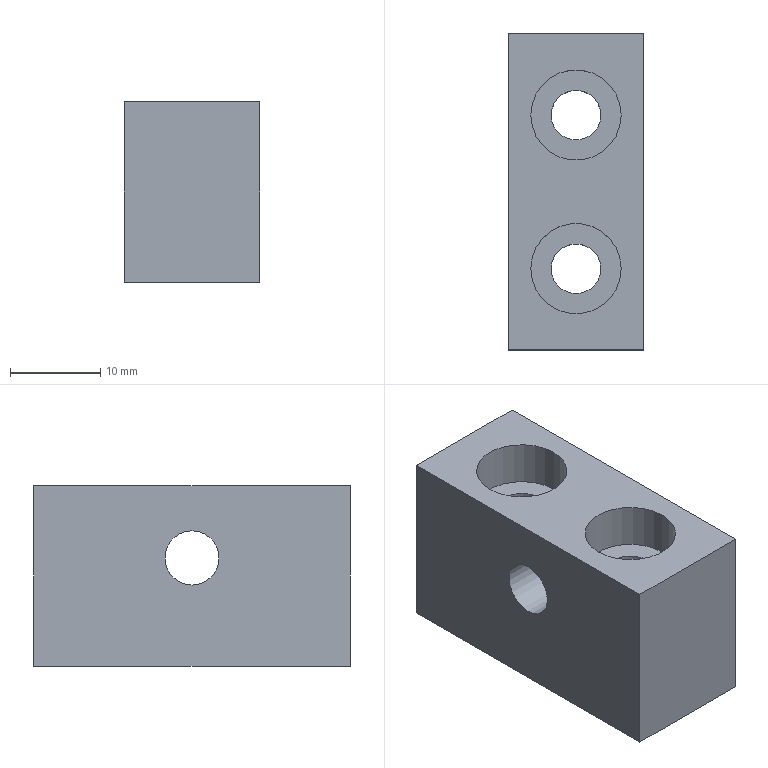Part | NX | features pneumatic support2 2 | 1 solid | 13 faces | box 15 x 35 x 20 mm | volume 8578 mm3 | plane 8 | cylinder 5 | commonest cylinder face diameters 5.5 x2 10 x2 6 x1
STEP:
#1=CARTESIAN_POINT('',(5.,8.5,15.));
#2=VERTEX_POINT('',#1);
#3=CARTESIAN_POINT('',(0.,8.5,15.));
#4=DIRECTION('',(0.,0.,1.));
#5=DIRECTION('',(1.,0.,0.));
#6=AXIS2_PLACEMENT_3D('',#3,#4,#5);
#7=CIRCLE('',#6,5.);
#8=EDGE_CURVE('',#2,#2,#7,.T.);
#9=ORIENTED_EDGE('',*,*,#8,.T.);
#10=EDGE_LOOP('',(#9));
#11=FACE_BOUND('',#10,.T.);
#12=CARTESIAN_POINT('',(2.75,8.5,15.));
#13=VERTEX_POINT('',#12);
#14=CARTESIAN_POINT('',(0.,8.5,15.));
#15=DIRECTION('',(0.,0.,1.));
#16=DIRECTION('',(1.,0.,0.));
#17=AXIS2_PLACEMENT_3D('',#14,#15,#16);
#18=CIRCLE('',#17,2.75);
#19=EDGE_CURVE('',#13,#13,#18,.F.);
#20=ORIENTED_EDGE('',*,*,#19,.T.);
#21=EDGE_LOOP('',(#20));
#22=FACE_BOUND('',#21,.T.);
#23=CARTESIAN_POINT('',(2.75,8.5,15.));
#24=DIRECTION('',(0.,0.,-1.));
#25=DIRECTION('',(-1.,0.,0.));
#26=AXIS2_PLACEMENT_3D('',#23,#24,#25);
#27=PLANE('',#26);
#28=ADVANCED_FACE('',(#11,#22),#27,.F.);
#29=CARTESIAN_POINT('',(5.,-8.5,15.));
#30=VERTEX_POINT('',#29);
#31=CARTESIAN_POINT('',(0.,-8.5,15.));
#32=DIRECTION('',(0.,0.,1.));
#33=DIRECTION('',(1.,0.,0.));
#34=AXIS2_PLACEMENT_3D('',#31,#32,#33);
#35=CIRCLE('',#34,5.);
#36=EDGE_CURVE('',#30,#30,#35,.T.);
#37=ORIENTED_EDGE('',*,*,#36,.T.);
#38=EDGE_LOOP('',(#37));
#39=FACE_BOUND('',#38,.T.);
#40=CARTESIAN_POINT('',(2.75,-8.5,15.));
#41=VERTEX_POINT('',#40);
#42=CARTESIAN_POINT('',(0.,-8.5,15.));
#43=DIRECTION('',(0.,0.,1.));
#44=DIRECTION('',(1.,0.,0.));
#45=AXIS2_PLACEMENT_3D('',#42,#43,#44);
#46=CIRCLE('',#45,2.75);
#47=EDGE_CURVE('',#41,#41,#46,.F.);
#48=ORIENTED_EDGE('',*,*,#47,.T.);
#49=EDGE_LOOP('',(#48));
#50=FACE_BOUND('',#49,.T.);
#51=CARTESIAN_POINT('',(2.75,-8.5,15.));
#52=DIRECTION('',(0.,0.,-1.));
#53=DIRECTION('',(-1.,0.,0.));
#54=AXIS2_PLACEMENT_3D('',#51,#52,#53);
#55=PLANE('',#54);
#56=ADVANCED_FACE('',(#39,#50),#55,.F.);
#57=ORIENTED_EDGE('',*,*,#8,.F.);
#58=EDGE_LOOP('',(#57));
#59=FACE_BOUND('',#58,.T.);
#60=CARTESIAN_POINT('',(5.,8.5,20.));
#61=VERTEX_POINT('',#60);
#62=CARTESIAN_POINT('',(0.,8.5,20.));
#63=DIRECTION('',(0.,0.,1.));
#64=DIRECTION('',(1.,0.,0.));
#65=AXIS2_PLACEMENT_3D('',#62,#63,#64);
#66=CIRCLE('',#65,5.);
#67=EDGE_CURVE('',#61,#61,#66,.T.);
#68=ORIENTED_EDGE('',*,*,#67,.T.);
#69=EDGE_LOOP('',(#68));
#70=FACE_BOUND('',#69,.T.);
#71=CARTESIAN_POINT('',(0.,8.5,20.));
#72=DIRECTION('',(0.,0.,1.));
#73=DIRECTION('',(1.,0.,0.));
#74=AXIS2_PLACEMENT_3D('',#71,#72,#73);
#75=CYLINDRICAL_SURFACE('',#74,5.);
#76=ADVANCED_FACE('',(#59,#70),#75,.F.);
#77=ORIENTED_EDGE('',*,*,#36,.F.);
#78=EDGE_LOOP('',(#77));
#79=FACE_BOUND('',#78,.T.);
#80=CARTESIAN_POINT('',(5.,-8.5,20.));
#81=VERTEX_POINT('',#80);
#82=CARTESIAN_POINT('',(0.,-8.5,20.));
#83=DIRECTION('',(0.,0.,1.));
#84=DIRECTION('',(1.,0.,0.));
#85=AXIS2_PLACEMENT_3D('',#82,#83,#84);
#86=CIRCLE('',#85,5.);
#87=EDGE_CURVE('',#81,#81,#86,.T.);
#88=ORIENTED_EDGE('',*,*,#87,.T.);
#89=EDGE_LOOP('',(#88));
#90=FACE_BOUND('',#89,.T.);
#91=CARTESIAN_POINT('',(0.,-8.5,20.));
#92=DIRECTION('',(0.,0.,1.));
#93=DIRECTION('',(1.,0.,0.));
#94=AXIS2_PLACEMENT_3D('',#91,#92,#93);
#95=CYLINDRICAL_SURFACE('',#94,5.);
#96=ADVANCED_FACE('',(#79,#90),#95,.F.);
#97=ORIENTED_EDGE('',*,*,#19,.F.);
#98=EDGE_LOOP('',(#97));
#99=FACE_BOUND('',#98,.T.);
#100=CARTESIAN_POINT('',(2.75,8.5,0.));
#101=VERTEX_POINT('',#100);
#102=CARTESIAN_POINT('',(0.,8.5,0.));
#103=DIRECTION('',(0.,0.,1.));
#104=DIRECTION('',(1.,0.,0.));
#105=AXIS2_PLACEMENT_3D('',#102,#103,#104);
#106=CIRCLE('',#105,2.75);
#107=EDGE_CURVE('',#101,#101,#106,.T.);
#108=ORIENTED_EDGE('',*,*,#107,.F.);
#109=EDGE_LOOP('',(#108));
#110=FACE_BOUND('',#109,.T.);
#111=CARTESIAN_POINT('',(0.,8.5,20.));
#112=DIRECTION('',(0.,0.,1.));
#113=DIRECTION('',(1.,0.,0.));
#114=AXIS2_PLACEMENT_3D('',#111,#112,#113);
#115=CYLINDRICAL_SURFACE('',#114,2.75);
#116=ADVANCED_FACE('',(#99,#110),#115,.F.);
#117=ORIENTED_EDGE('',*,*,#47,.F.);
#118=EDGE_LOOP('',(#117));
#119=FACE_BOUND('',#118,.T.);
#120=CARTESIAN_POINT('',(2.75,-8.5,0.));
#121=VERTEX_POINT('',#120);
#122=CARTESIAN_POINT('',(0.,-8.5,0.));
#123=DIRECTION('',(0.,0.,1.));
#124=DIRECTION('',(1.,0.,0.));
#125=AXIS2_PLACEMENT_3D('',#122,#123,#124);
#126=CIRCLE('',#125,2.75);
#127=EDGE_CURVE('',#121,#121,#126,.T.);
#128=ORIENTED_EDGE('',*,*,#127,.F.);
#129=EDGE_LOOP('',(#128));
#130=FACE_BOUND('',#129,.T.);
#131=CARTESIAN_POINT('',(0.,-8.5,20.));
#132=DIRECTION('',(0.,0.,1.));
#133=DIRECTION('',(1.,0.,0.));
#134=AXIS2_PLACEMENT_3D('',#131,#132,#133);
#135=CYLINDRICAL_SURFACE('',#134,2.75);
#136=ADVANCED_FACE('',(#119,#130),#135,.F.);
#137=CARTESIAN_POINT('',(7.5,17.5,0.));
#138=VERTEX_POINT('',#137);
#139=CARTESIAN_POINT('',(7.5,17.5,20.));
#140=VERTEX_POINT('',#139);
#141=CARTESIAN_POINT('',(7.5,17.5,20.));
#142=DIRECTION('',(0.,0.,-1.));
#143=VECTOR('',#142,1000.);
#144=LINE('',#141,#143);
#145=EDGE_CURVE('',#138,#140,#144,.F.);
#146=ORIENTED_EDGE('',*,*,#145,.T.);
#147=CARTESIAN_POINT('',(7.5,-17.5,20.));
#148=VERTEX_POINT('',#147);
#149=CARTESIAN_POINT('',(7.5,17.5,20.));
#150=DIRECTION('',(0.,1.,0.));
#151=VECTOR('',#150,1000.);
#152=LINE('',#149,#151);
#153=EDGE_CURVE('',#140,#148,#152,.F.);
#154=ORIENTED_EDGE('',*,*,#153,.T.);
#155=CARTESIAN_POINT('',(7.5,-17.5,0.));
#156=VERTEX_POINT('',#155);
#157=CARTESIAN_POINT('',(7.5,-17.5,20.));
#158=DIRECTION('',(0.,0.,1.));
#159=VECTOR('',#158,1000.);
#160=LINE('',#157,#159);
#161=EDGE_CURVE('',#148,#156,#160,.F.);
#162=ORIENTED_EDGE('',*,*,#161,.T.);
#163=CARTESIAN_POINT('',(7.5,17.5,0.));
#164=DIRECTION('',(0.,1.,0.));
#165=VECTOR('',#164,1000.);
#166=LINE('',#163,#165);
#167=EDGE_CURVE('',#138,#156,#166,.F.);
#168=ORIENTED_EDGE('',*,*,#167,.F.);
#169=EDGE_LOOP('',(#146,#154,#162,#168));
#170=FACE_BOUND('',#169,.T.);
#171=CARTESIAN_POINT('',(7.5,0.,9.));
#172=VERTEX_POINT('',#171);
#173=CARTESIAN_POINT('',(7.5,0.,12.));
#174=DIRECTION('',(1.,0.,0.));
#175=DIRECTION('',(0.,0.,-1.));
#176=AXIS2_PLACEMENT_3D('',#173,#174,#175);
#177=CIRCLE('',#176,3.);
#178=EDGE_CURVE('',#172,#172,#177,.F.);
#179=ORIENTED_EDGE('',*,*,#178,.T.);
#180=EDGE_LOOP('',(#179));
#181=FACE_BOUND('',#180,.T.);
#182=CARTESIAN_POINT('',(7.5,-17.5,20.));
#183=DIRECTION('',(-1.,0.,0.));
#184=DIRECTION('',(0.,0.,1.));
#185=AXIS2_PLACEMENT_3D('',#182,#183,#184);
#186=PLANE('',#185);
#187=ADVANCED_FACE('',(#170,#181),#186,.F.);
#188=CARTESIAN_POINT('',(-7.5,0.,9.));
#189=VERTEX_POINT('',#188);
#190=CARTESIAN_POINT('',(-7.5,0.,12.));
#191=DIRECTION('',(1.,0.,0.));
#192=DIRECTION('',(0.,0.,-1.));
#193=AXIS2_PLACEMENT_3D('',#190,#191,#192);
#194=CIRCLE('',#193,3.);
#195=EDGE_CURVE('',#189,#189,#194,.F.);
#196=ORIENTED_EDGE('',*,*,#195,.T.);
#197=EDGE_LOOP('',(#196));
#198=FACE_BOUND('',#197,.T.);
#199=ORIENTED_EDGE('',*,*,#178,.F.);
#200=EDGE_LOOP('',(#199));
#201=FACE_BOUND('',#200,.T.);
#202=CARTESIAN_POINT('',(-7.5,0.,12.));
#203=DIRECTION('',(1.,0.,0.));
#204=DIRECTION('',(0.,0.,-1.));
#205=AXIS2_PLACEMENT_3D('',#202,#203,#204);
#206=CYLINDRICAL_SURFACE('',#205,3.);
#207=ADVANCED_FACE('',(#198,#201),#206,.F.);
#208=CARTESIAN_POINT('',(-7.5,17.5,0.));
#209=VERTEX_POINT('',#208);
#210=CARTESIAN_POINT('',(-7.5,17.5,20.));
#211=VERTEX_POINT('',#210);
#212=CARTESIAN_POINT('',(-7.5,17.5,20.));
#213=DIRECTION('',(0.,0.,-1.));
#214=VECTOR('',#213,1000.);
#215=LINE('',#212,#214);
#216=EDGE_CURVE('',#209,#211,#215,.F.);
#217=ORIENTED_EDGE('',*,*,#216,.T.);
#218=CARTESIAN_POINT('',(7.5,17.5,20.));
#219=DIRECTION('',(-1.,0.,0.));
#220=VECTOR('',#219,1000.);
#221=LINE('',#218,#220);
#222=EDGE_CURVE('',#211,#140,#221,.F.);
#223=ORIENTED_EDGE('',*,*,#222,.T.);
#224=ORIENTED_EDGE('',*,*,#145,.F.);
#225=CARTESIAN_POINT('',(7.5,17.5,0.));
#226=DIRECTION('',(-1.,0.,0.));
#227=VECTOR('',#226,1000.);
#228=LINE('',#225,#227);
#229=EDGE_CURVE('',#209,#138,#228,.F.);
#230=ORIENTED_EDGE('',*,*,#229,.F.);
#231=EDGE_LOOP('',(#217,#223,#224,#230));
#232=FACE_BOUND('',#231,.T.);
#233=CARTESIAN_POINT('',(-7.5,17.5,20.));
#234=DIRECTION('',(0.,-1.,0.));
#235=DIRECTION('',(0.,0.,-1.));
#236=AXIS2_PLACEMENT_3D('',#233,#234,#235);
#237=PLANE('',#236);
#238=ADVANCED_FACE('',(#232),#237,.F.);
#239=ORIENTED_EDGE('',*,*,#222,.F.);
#240=CARTESIAN_POINT('',(-7.5,-17.5,20.));
#241=VERTEX_POINT('',#240);
#242=CARTESIAN_POINT('',(-7.5,-17.5,20.));
#243=DIRECTION('',(0.,1.,0.));
#244=VECTOR('',#243,1000.);
#245=LINE('',#242,#244);
#246=EDGE_CURVE('',#211,#241,#245,.F.);
#247=ORIENTED_EDGE('',*,*,#246,.T.);
#248=CARTESIAN_POINT('',(-7.5,-17.5,20.));
#249=DIRECTION('',(1.,0.,0.));
#250=VECTOR('',#249,1000.);
#251=LINE('',#248,#250);
#252=EDGE_CURVE('',#241,#148,#251,.T.);
#253=ORIENTED_EDGE('',*,*,#252,.T.);
#254=ORIENTED_EDGE('',*,*,#153,.F.);
#255=EDGE_LOOP('',(#239,#247,#253,#254));
#256=FACE_BOUND('',#255,.T.);
#257=ORIENTED_EDGE('',*,*,#87,.F.);
#258=EDGE_LOOP('',(#257));
#259=FACE_BOUND('',#258,.T.);
#260=ORIENTED_EDGE('',*,*,#67,.F.);
#261=EDGE_LOOP('',(#260));
#262=FACE_BOUND('',#261,.T.);
#263=CARTESIAN_POINT('',(7.5,17.5,20.));
#264=DIRECTION('',(0.,0.,-1.));
#265=DIRECTION('',(-1.,0.,0.));
#266=AXIS2_PLACEMENT_3D('',#263,#264,#265);
#267=PLANE('',#266);
#268=ADVANCED_FACE('',(#256,#259,#262),#267,.F.);
#269=ORIENTED_EDGE('',*,*,#161,.F.);
#270=ORIENTED_EDGE('',*,*,#252,.F.);
#271=CARTESIAN_POINT('',(-7.5,-17.5,0.));
#272=VERTEX_POINT('',#271);
#273=CARTESIAN_POINT('',(-7.5,-17.5,20.));
#274=DIRECTION('',(0.,0.,-1.));
#275=VECTOR('',#274,1000.);
#276=LINE('',#273,#275);
#277=EDGE_CURVE('',#241,#272,#276,.T.);
#278=ORIENTED_EDGE('',*,*,#277,.T.);
#279=CARTESIAN_POINT('',(7.5,-17.5,0.));
#280=DIRECTION('',(-1.,0.,0.));
#281=VECTOR('',#280,1000.);
#282=LINE('',#279,#281);
#283=EDGE_CURVE('',#156,#272,#282,.T.);
#284=ORIENTED_EDGE('',*,*,#283,.F.);
#285=EDGE_LOOP('',(#269,#270,#278,#284));
#286=FACE_BOUND('',#285,.T.);
#287=CARTESIAN_POINT('',(-7.5,-17.5,20.));
#288=DIRECTION('',(0.,1.,0.));
#289=DIRECTION('',(0.,0.,1.));
#290=AXIS2_PLACEMENT_3D('',#287,#288,#289);
#291=PLANE('',#290);
#292=ADVANCED_FACE('',(#286),#291,.F.);
#293=CARTESIAN_POINT('',(-7.5,-17.5,0.));
#294=DIRECTION('',(0.,1.,0.));
#295=VECTOR('',#294,1000.);
#296=LINE('',#293,#295);
#297=EDGE_CURVE('',#272,#209,#296,.T.);
#298=ORIENTED_EDGE('',*,*,#297,.T.);
#299=ORIENTED_EDGE('',*,*,#229,.T.);
#300=ORIENTED_EDGE('',*,*,#167,.T.);
#301=ORIENTED_EDGE('',*,*,#283,.T.);
#302=EDGE_LOOP('',(#298,#299,#300,#301));
#303=FACE_BOUND('',#302,.T.);
#304=ORIENTED_EDGE('',*,*,#127,.T.);
#305=EDGE_LOOP('',(#304));
#306=FACE_BOUND('',#305,.T.);
#307=ORIENTED_EDGE('',*,*,#107,.T.);
#308=EDGE_LOOP('',(#307));
#309=FACE_BOUND('',#308,.T.);
#310=CARTESIAN_POINT('',(7.5,17.5,0.));
#311=DIRECTION('',(0.,0.,-1.));
#312=DIRECTION('',(-1.,0.,0.));
#313=AXIS2_PLACEMENT_3D('',#310,#311,#312);
#314=PLANE('',#313);
#315=ADVANCED_FACE('',(#303,#306,#309),#314,.T.);
#316=ORIENTED_EDGE('',*,*,#277,.F.);
#317=ORIENTED_EDGE('',*,*,#246,.F.);
#318=ORIENTED_EDGE('',*,*,#216,.F.);
#319=ORIENTED_EDGE('',*,*,#297,.F.);
#320=EDGE_LOOP('',(#316,#317,#318,#319));
#321=FACE_BOUND('',#320,.T.);
#322=ORIENTED_EDGE('',*,*,#195,.F.);
#323=EDGE_LOOP('',(#322));
#324=FACE_BOUND('',#323,.T.);
#325=CARTESIAN_POINT('',(-7.5,-17.5,20.));
#326=DIRECTION('',(1.,0.,0.));
#327=DIRECTION('',(0.,0.,-1.));
#328=AXIS2_PLACEMENT_3D('',#325,#326,#327);
#329=PLANE('',#328);
#330=ADVANCED_FACE('',(#321,#324),#329,.F.);
#331=CLOSED_SHELL('',(#28,#56,#76,#96,#116,#136,#187,#207,#238,#268,#292,#315,#330));
#332=MANIFOLD_SOLID_BREP('',#331);
#333=(LENGTH_UNIT()NAMED_UNIT(*)SI_UNIT(.MILLI.,.METRE.));
#334=UNCERTAINTY_MEASURE_WITH_UNIT(LENGTH_MEASURE(0.00001),#333,'','');
#335=(NAMED_UNIT(*)PLANE_ANGLE_UNIT()SI_UNIT($,.RADIAN.));
#336=(NAMED_UNIT(*)SI_UNIT($,.STERADIAN.)SOLID_ANGLE_UNIT());
#337=(GEOMETRIC_REPRESENTATION_CONTEXT(3)GLOBAL_UNCERTAINTY_ASSIGNED_CONTEXT((#334))GLOBAL_UNIT_ASSIGNED_CONTEXT((#333,#335,#336))REPRESENTATION_CONTEXT('',''));
#338=ADVANCED_BREP_SHAPE_REPRESENTATION('',(#332),#337);